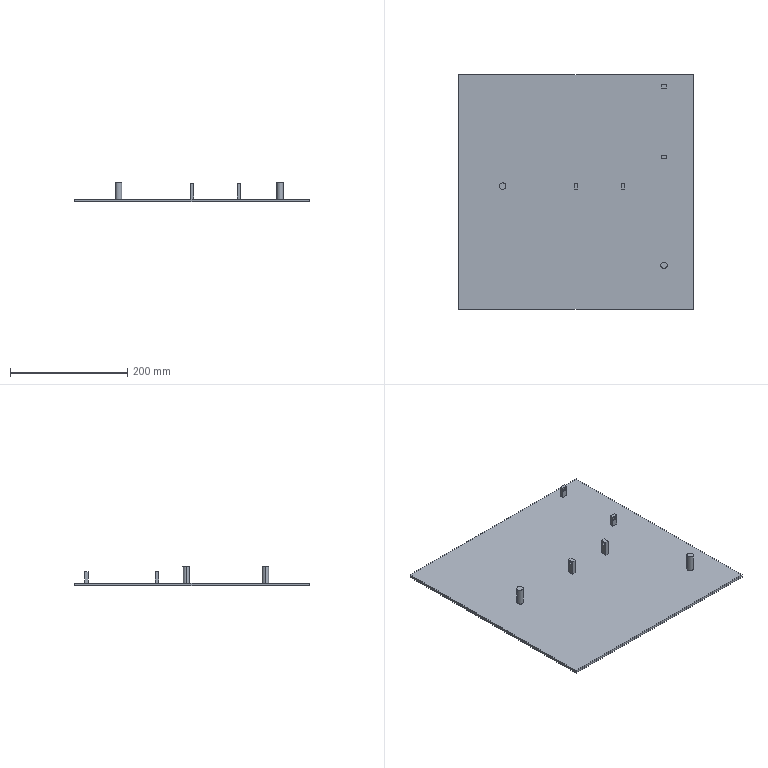Part | SolidWorks | features ICE 6, Extrusion 1 | 1 solid | 66 faces | box 400 x 400 x 34 mm | volume 809134 mm3 | plane 50 | cylinder 16 | commonest cylinder face diameters 5 x8 10 x4 11 x4